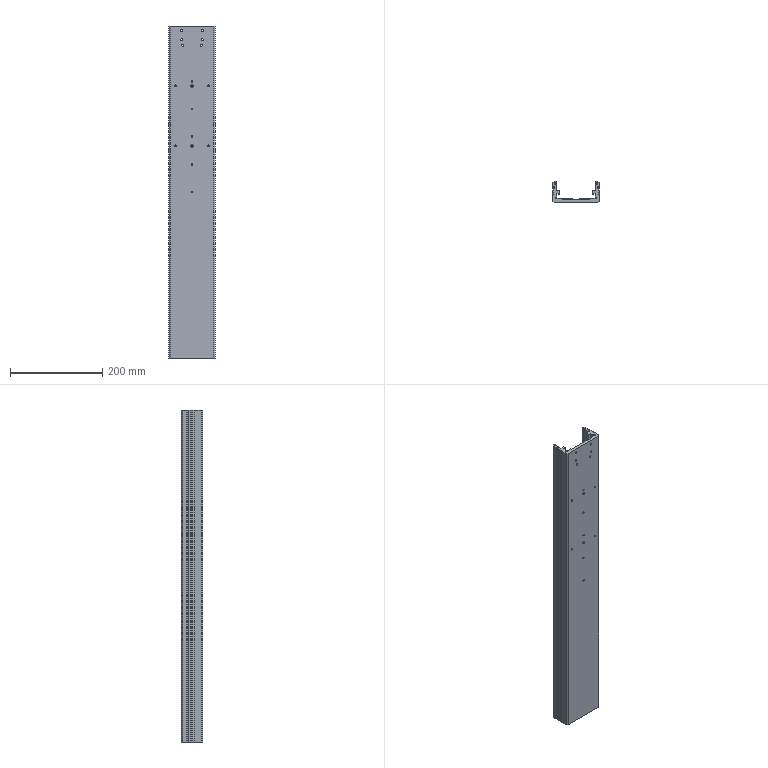Part | NX | 1 solid | 107 faces | box 100 x 46 x 720 mm | volume 991013 mm3 | plane 62 | cylinder 45 | commonest cylinder face diameters 0.6 x18 4.2 x10 3.3 x5 3.2 x4 0.4 x2 4 x2